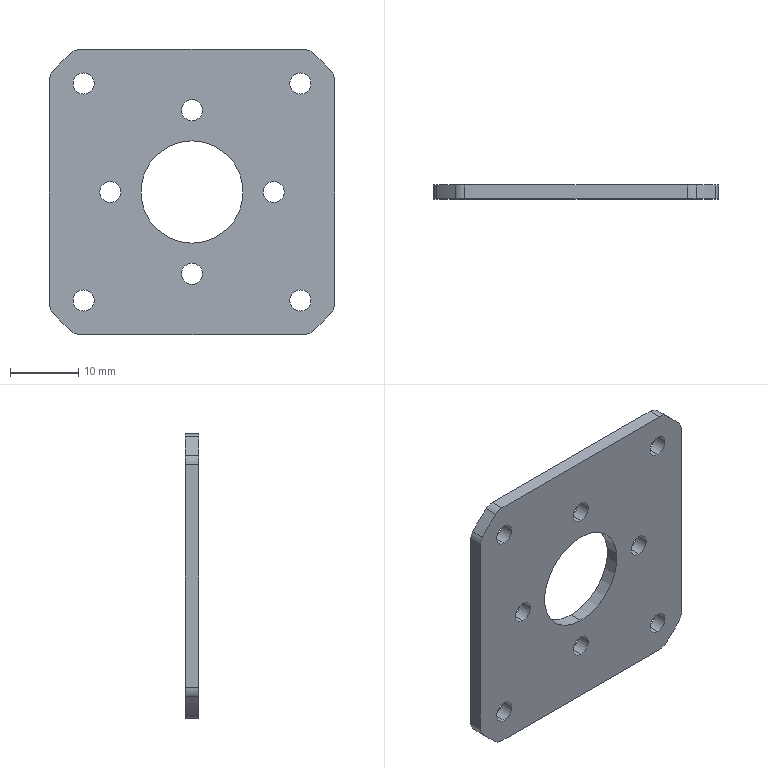Part | SolidWorks | features Extrusion 1, Fillet 1 | 1 solid | 36 faces | box 41.82 x 2 x 41.82 mm | volume 2968 mm3 | cylinder 30 | plane 6 | commonest cylinder face diameters 3.1 x16 4 x8 54 x4 15 x2
STEP:
#1=CARTESIAN_POINT('',(-15.91,2.,-17.46));
#2=VERTEX_POINT('',#1);
#3=CARTESIAN_POINT('',(-15.91,2.,-14.36));
#4=VERTEX_POINT('',#3);
#5=CARTESIAN_POINT('',(-15.91,2.,-15.91));
#6=DIRECTION('',(0.,1.,0.));
#7=DIRECTION('',(0.,0.,1.));
#8=AXIS2_PLACEMENT_3D('',#5,#6,#7);
#9=CIRCLE('',#8,1.55);
#10=EDGE_CURVE('',#2,#4,#9,.T.);
#11=ORIENTED_EDGE('',*,*,#10,.T.);
#12=CARTESIAN_POINT('',(-15.91,0.,-14.36));
#13=VERTEX_POINT('',#12);
#14=CARTESIAN_POINT('',(-15.91,2.,-14.36));
#15=DIRECTION('',(0.,-1.,0.));
#16=VECTOR('',#15,1000.);
#17=LINE('',#14,#16);
#18=EDGE_CURVE('',#4,#13,#17,.T.);
#19=ORIENTED_EDGE('',*,*,#18,.T.);
#20=CARTESIAN_POINT('',(-15.91,0.,-17.46));
#21=VERTEX_POINT('',#20);
#22=CARTESIAN_POINT('',(-15.91,0.,-15.91));
#23=DIRECTION('',(0.,1.,0.));
#24=DIRECTION('',(0.,0.,1.));
#25=AXIS2_PLACEMENT_3D('',#22,#23,#24);
#26=CIRCLE('',#25,1.55);
#27=EDGE_CURVE('',#21,#13,#26,.T.);
#28=ORIENTED_EDGE('',*,*,#27,.F.);
#29=CARTESIAN_POINT('',(-15.91,2.,-17.46));
#30=DIRECTION('',(0.,-1.,0.));
#31=VECTOR('',#30,1000.);
#32=LINE('',#29,#31);
#33=EDGE_CURVE('',#2,#21,#32,.T.);
#34=ORIENTED_EDGE('',*,*,#33,.F.);
#35=EDGE_LOOP('',(#11,#19,#28,#34));
#36=FACE_OUTER_BOUND('',#35,.T.);
#37=CARTESIAN_POINT('',(-15.91,2.,-15.91));
#38=DIRECTION('',(0.,-1.,0.));
#39=DIRECTION('',(0.,0.,-1.));
#40=AXIS2_PLACEMENT_3D('',#37,#38,#39);
#41=CYLINDRICAL_SURFACE('',#40,1.55);
#42=ADVANCED_FACE('',(#36),#41,.F.);
#43=CARTESIAN_POINT('',(0.,2.,-13.55));
#44=VERTEX_POINT('',#43);
#45=CARTESIAN_POINT('',(0.,2.,-10.45));
#46=VERTEX_POINT('',#45);
#47=CARTESIAN_POINT('',(0.,2.,-12.));
#48=DIRECTION('',(0.,1.,0.));
#49=DIRECTION('',(0.,0.,1.));
#50=AXIS2_PLACEMENT_3D('',#47,#48,#49);
#51=CIRCLE('',#50,1.55);
#52=EDGE_CURVE('',#44,#46,#51,.T.);
#53=ORIENTED_EDGE('',*,*,#52,.T.);
#54=CARTESIAN_POINT('',(0.,0.,-10.45));
#55=VERTEX_POINT('',#54);
#56=CARTESIAN_POINT('',(0.,2.,-10.45));
#57=DIRECTION('',(0.,-1.,0.));
#58=VECTOR('',#57,1000.);
#59=LINE('',#56,#58);
#60=EDGE_CURVE('',#46,#55,#59,.T.);
#61=ORIENTED_EDGE('',*,*,#60,.T.);
#62=CARTESIAN_POINT('',(0.,0.,-13.55));
#63=VERTEX_POINT('',#62);
#64=CARTESIAN_POINT('',(0.,0.,-12.));
#65=DIRECTION('',(0.,1.,0.));
#66=DIRECTION('',(0.,0.,1.));
#67=AXIS2_PLACEMENT_3D('',#64,#65,#66);
#68=CIRCLE('',#67,1.55);
#69=EDGE_CURVE('',#63,#55,#68,.T.);
#70=ORIENTED_EDGE('',*,*,#69,.F.);
#71=CARTESIAN_POINT('',(0.,2.,-13.55));
#72=DIRECTION('',(0.,-1.,0.));
#73=VECTOR('',#72,1000.);
#74=LINE('',#71,#73);
#75=EDGE_CURVE('',#44,#63,#74,.T.);
#76=ORIENTED_EDGE('',*,*,#75,.F.);
#77=EDGE_LOOP('',(#53,#61,#70,#76));
#78=FACE_OUTER_BOUND('',#77,.T.);
#79=CARTESIAN_POINT('',(0.,2.,-12.));
#80=DIRECTION('',(0.,-1.,0.));
#81=DIRECTION('',(0.,0.,-1.));
#82=AXIS2_PLACEMENT_3D('',#79,#80,#81);
#83=CYLINDRICAL_SURFACE('',#82,1.55);
#84=ADVANCED_FACE('',(#78),#83,.F.);
#85=CARTESIAN_POINT('',(-15.91,2.,14.36));
#86=VERTEX_POINT('',#85);
#87=CARTESIAN_POINT('',(-15.91,2.,17.46));
#88=VERTEX_POINT('',#87);
#89=CARTESIAN_POINT('',(-15.91,2.,15.91));
#90=DIRECTION('',(0.,1.,0.));
#91=DIRECTION('',(0.,0.,1.));
#92=AXIS2_PLACEMENT_3D('',#89,#90,#91);
#93=CIRCLE('',#92,1.55);
#94=EDGE_CURVE('',#86,#88,#93,.T.);
#95=ORIENTED_EDGE('',*,*,#94,.T.);
#96=CARTESIAN_POINT('',(-15.91,0.,17.46));
#97=VERTEX_POINT('',#96);
#98=CARTESIAN_POINT('',(-15.91,2.,17.46));
#99=DIRECTION('',(0.,-1.,0.));
#100=VECTOR('',#99,1000.);
#101=LINE('',#98,#100);
#102=EDGE_CURVE('',#88,#97,#101,.T.);
#103=ORIENTED_EDGE('',*,*,#102,.T.);
#104=CARTESIAN_POINT('',(-15.91,0.,14.36));
#105=VERTEX_POINT('',#104);
#106=CARTESIAN_POINT('',(-15.91,0.,15.91));
#107=DIRECTION('',(0.,1.,0.));
#108=DIRECTION('',(0.,0.,1.));
#109=AXIS2_PLACEMENT_3D('',#106,#107,#108);
#110=CIRCLE('',#109,1.55);
#111=EDGE_CURVE('',#105,#97,#110,.T.);
#112=ORIENTED_EDGE('',*,*,#111,.F.);
#113=CARTESIAN_POINT('',(-15.91,2.,14.36));
#114=DIRECTION('',(0.,-1.,0.));
#115=VECTOR('',#114,1000.);
#116=LINE('',#113,#115);
#117=EDGE_CURVE('',#86,#105,#116,.T.);
#118=ORIENTED_EDGE('',*,*,#117,.F.);
#119=EDGE_LOOP('',(#95,#103,#112,#118));
#120=FACE_OUTER_BOUND('',#119,.T.);
#121=CARTESIAN_POINT('',(-15.91,2.,15.91));
#122=DIRECTION('',(0.,-1.,0.));
#123=DIRECTION('',(0.,0.,-1.));
#124=AXIS2_PLACEMENT_3D('',#121,#122,#123);
#125=CYLINDRICAL_SURFACE('',#124,1.55);
#126=ADVANCED_FACE('',(#120),#125,.F.);
#127=CARTESIAN_POINT('',(-12.,2.,-1.55));
#128=VERTEX_POINT('',#127);
#129=CARTESIAN_POINT('',(-12.,2.,1.55));
#130=VERTEX_POINT('',#129);
#131=CARTESIAN_POINT('',(-12.,2.,0.));
#132=DIRECTION('',(0.,1.,0.));
#133=DIRECTION('',(0.,0.,1.));
#134=AXIS2_PLACEMENT_3D('',#131,#132,#133);
#135=CIRCLE('',#134,1.55);
#136=EDGE_CURVE('',#128,#130,#135,.T.);
#137=ORIENTED_EDGE('',*,*,#136,.T.);
#138=CARTESIAN_POINT('',(-12.,0.,1.55));
#139=VERTEX_POINT('',#138);
#140=CARTESIAN_POINT('',(-12.,2.,1.55));
#141=DIRECTION('',(0.,-1.,0.));
#142=VECTOR('',#141,1000.);
#143=LINE('',#140,#142);
#144=EDGE_CURVE('',#130,#139,#143,.T.);
#145=ORIENTED_EDGE('',*,*,#144,.T.);
#146=CARTESIAN_POINT('',(-12.,0.,-1.55));
#147=VERTEX_POINT('',#146);
#148=CARTESIAN_POINT('',(-12.,0.,0.));
#149=DIRECTION('',(0.,1.,0.));
#150=DIRECTION('',(0.,0.,1.));
#151=AXIS2_PLACEMENT_3D('',#148,#149,#150);
#152=CIRCLE('',#151,1.55);
#153=EDGE_CURVE('',#147,#139,#152,.T.);
#154=ORIENTED_EDGE('',*,*,#153,.F.);
#155=CARTESIAN_POINT('',(-12.,2.,-1.55));
#156=DIRECTION('',(0.,-1.,0.));
#157=VECTOR('',#156,1000.);
#158=LINE('',#155,#157);
#159=EDGE_CURVE('',#128,#147,#158,.T.);
#160=ORIENTED_EDGE('',*,*,#159,.F.);
#161=EDGE_LOOP('',(#137,#145,#154,#160));
#162=FACE_OUTER_BOUND('',#161,.T.);
#163=CARTESIAN_POINT('',(-12.,2.,0.));
#164=DIRECTION('',(0.,-1.,0.));
#165=DIRECTION('',(0.,0.,-1.));
#166=AXIS2_PLACEMENT_3D('',#163,#164,#165);
#167=CYLINDRICAL_SURFACE('',#166,1.55);
#168=ADVANCED_FACE('',(#162),#167,.F.);
#169=CARTESIAN_POINT('',(15.91,2.,14.36));
#170=VERTEX_POINT('',#169);
#171=CARTESIAN_POINT('',(15.91,2.,17.46));
#172=VERTEX_POINT('',#171);
#173=CARTESIAN_POINT('',(15.91,2.,15.91));
#174=DIRECTION('',(0.,1.,0.));
#175=DIRECTION('',(0.,0.,1.));
#176=AXIS2_PLACEMENT_3D('',#173,#174,#175);
#177=CIRCLE('',#176,1.55);
#178=EDGE_CURVE('',#170,#172,#177,.T.);
#179=ORIENTED_EDGE('',*,*,#178,.T.);
#180=CARTESIAN_POINT('',(15.91,0.,17.46));
#181=VERTEX_POINT('',#180);
#182=CARTESIAN_POINT('',(15.91,2.,17.46));
#183=DIRECTION('',(0.,-1.,0.));
#184=VECTOR('',#183,1000.);
#185=LINE('',#182,#184);
#186=EDGE_CURVE('',#172,#181,#185,.T.);
#187=ORIENTED_EDGE('',*,*,#186,.T.);
#188=CARTESIAN_POINT('',(15.91,0.,14.36));
#189=VERTEX_POINT('',#188);
#190=CARTESIAN_POINT('',(15.91,0.,15.91));
#191=DIRECTION('',(0.,1.,0.));
#192=DIRECTION('',(0.,0.,1.));
#193=AXIS2_PLACEMENT_3D('',#190,#191,#192);
#194=CIRCLE('',#193,1.55);
#195=EDGE_CURVE('',#189,#181,#194,.T.);
#196=ORIENTED_EDGE('',*,*,#195,.F.);
#197=CARTESIAN_POINT('',(15.91,2.,14.36));
#198=DIRECTION('',(0.,-1.,0.));
#199=VECTOR('',#198,1000.);
#200=LINE('',#197,#199);
#201=EDGE_CURVE('',#170,#189,#200,.T.);
#202=ORIENTED_EDGE('',*,*,#201,.F.);
#203=EDGE_LOOP('',(#179,#187,#196,#202));
#204=FACE_OUTER_BOUND('',#203,.T.);
#205=CARTESIAN_POINT('',(15.91,2.,15.91));
#206=DIRECTION('',(0.,-1.,0.));
#207=DIRECTION('',(0.,0.,-1.));
#208=AXIS2_PLACEMENT_3D('',#205,#206,#207);
#209=CYLINDRICAL_SURFACE('',#208,1.55);
#210=ADVANCED_FACE('',(#204),#209,.F.);
#211=CARTESIAN_POINT('',(0.,2.,10.45));
#212=VERTEX_POINT('',#211);
#213=CARTESIAN_POINT('',(0.,2.,13.55));
#214=VERTEX_POINT('',#213);
#215=CARTESIAN_POINT('',(0.,2.,12.));
#216=DIRECTION('',(0.,1.,0.));
#217=DIRECTION('',(0.,0.,1.));
#218=AXIS2_PLACEMENT_3D('',#215,#216,#217);
#219=CIRCLE('',#218,1.55);
#220=EDGE_CURVE('',#212,#214,#219,.T.);
#221=ORIENTED_EDGE('',*,*,#220,.T.);
#222=CARTESIAN_POINT('',(0.,0.,13.55));
#223=VERTEX_POINT('',#222);
#224=CARTESIAN_POINT('',(0.,2.,13.55));
#225=DIRECTION('',(0.,-1.,0.));
#226=VECTOR('',#225,1000.);
#227=LINE('',#224,#226);
#228=EDGE_CURVE('',#214,#223,#227,.T.);
#229=ORIENTED_EDGE('',*,*,#228,.T.);
#230=CARTESIAN_POINT('',(0.,0.,10.45));
#231=VERTEX_POINT('',#230);
#232=CARTESIAN_POINT('',(0.,0.,12.));
#233=DIRECTION('',(0.,1.,0.));
#234=DIRECTION('',(0.,0.,1.));
#235=AXIS2_PLACEMENT_3D('',#232,#233,#234);
#236=CIRCLE('',#235,1.55);
#237=EDGE_CURVE('',#231,#223,#236,.T.);
#238=ORIENTED_EDGE('',*,*,#237,.F.);
#239=CARTESIAN_POINT('',(0.,2.,10.45));
#240=DIRECTION('',(0.,-1.,0.));
#241=VECTOR('',#240,1000.);
#242=LINE('',#239,#241);
#243=EDGE_CURVE('',#212,#231,#242,.T.);
#244=ORIENTED_EDGE('',*,*,#243,.F.);
#245=EDGE_LOOP('',(#221,#229,#238,#244));
#246=FACE_OUTER_BOUND('',#245,.T.);
#247=CARTESIAN_POINT('',(0.,2.,12.));
#248=DIRECTION('',(0.,-1.,0.));
#249=DIRECTION('',(0.,0.,-1.));
#250=AXIS2_PLACEMENT_3D('',#247,#248,#249);
#251=CYLINDRICAL_SURFACE('',#250,1.55);
#252=ADVANCED_FACE('',(#246),#251,.F.);
#253=CARTESIAN_POINT('',(15.91,2.,-17.46));
#254=VERTEX_POINT('',#253);
#255=CARTESIAN_POINT('',(15.91,2.,-14.36));
#256=VERTEX_POINT('',#255);
#257=CARTESIAN_POINT('',(15.91,2.,-15.91));
#258=DIRECTION('',(0.,1.,0.));
#259=DIRECTION('',(0.,0.,1.));
#260=AXIS2_PLACEMENT_3D('',#257,#258,#259);
#261=CIRCLE('',#260,1.55);
#262=EDGE_CURVE('',#254,#256,#261,.T.);
#263=ORIENTED_EDGE('',*,*,#262,.T.);
#264=CARTESIAN_POINT('',(15.91,0.,-14.36));
#265=VERTEX_POINT('',#264);
#266=CARTESIAN_POINT('',(15.91,2.,-14.36));
#267=DIRECTION('',(0.,-1.,0.));
#268=VECTOR('',#267,1000.);
#269=LINE('',#266,#268);
#270=EDGE_CURVE('',#256,#265,#269,.T.);
#271=ORIENTED_EDGE('',*,*,#270,.T.);
#272=CARTESIAN_POINT('',(15.91,0.,-17.46));
#273=VERTEX_POINT('',#272);
#274=CARTESIAN_POINT('',(15.91,0.,-15.91));
#275=DIRECTION('',(0.,1.,0.));
#276=DIRECTION('',(0.,0.,1.));
#277=AXIS2_PLACEMENT_3D('',#274,#275,#276);
#278=CIRCLE('',#277,1.55);
#279=EDGE_CURVE('',#273,#265,#278,.T.);
#280=ORIENTED_EDGE('',*,*,#279,.F.);
#281=CARTESIAN_POINT('',(15.91,2.,-17.46));
#282=DIRECTION('',(0.,-1.,0.));
#283=VECTOR('',#282,1000.);
#284=LINE('',#281,#283);
#285=EDGE_CURVE('',#254,#273,#284,.T.);
#286=ORIENTED_EDGE('',*,*,#285,.F.);
#287=EDGE_LOOP('',(#263,#271,#280,#286));
#288=FACE_OUTER_BOUND('',#287,.T.);
#289=CARTESIAN_POINT('',(15.91,2.,-15.91));
#290=DIRECTION('',(0.,-1.,0.));
#291=DIRECTION('',(0.,0.,-1.));
#292=AXIS2_PLACEMENT_3D('',#289,#290,#291);
#293=CYLINDRICAL_SURFACE('',#292,1.55);
#294=ADVANCED_FACE('',(#288),#293,.F.);
#295=CARTESIAN_POINT('',(12.,2.,-1.55));
#296=VERTEX_POINT('',#295);
#297=CARTESIAN_POINT('',(12.,2.,1.55));
#298=VERTEX_POINT('',#297);
#299=CARTESIAN_POINT('',(12.,2.,0.));
#300=DIRECTION('',(0.,1.,0.));
#301=DIRECTION('',(0.,0.,1.));
#302=AXIS2_PLACEMENT_3D('',#299,#300,#301);
#303=CIRCLE('',#302,1.55);
#304=EDGE_CURVE('',#296,#298,#303,.T.);
#305=ORIENTED_EDGE('',*,*,#304,.T.);
#306=CARTESIAN_POINT('',(12.,0.,1.55));
#307=VERTEX_POINT('',#306);
#308=CARTESIAN_POINT('',(12.,2.,1.55));
#309=DIRECTION('',(0.,-1.,0.));
#310=VECTOR('',#309,1000.);
#311=LINE('',#308,#310);
#312=EDGE_CURVE('',#298,#307,#311,.T.);
#313=ORIENTED_EDGE('',*,*,#312,.T.);
#314=CARTESIAN_POINT('',(12.,0.,-1.55));
#315=VERTEX_POINT('',#314);
#316=CARTESIAN_POINT('',(12.,0.,0.));
#317=DIRECTION('',(0.,1.,0.));
#318=DIRECTION('',(0.,0.,1.));
#319=AXIS2_PLACEMENT_3D('',#316,#317,#318);
#320=CIRCLE('',#319,1.55);
#321=EDGE_CURVE('',#315,#307,#320,.T.);
#322=ORIENTED_EDGE('',*,*,#321,.F.);
#323=CARTESIAN_POINT('',(12.,2.,-1.55));
#324=DIRECTION('',(0.,-1.,0.));
#325=VECTOR('',#324,1000.);
#326=LINE('',#323,#325);
#327=EDGE_CURVE('',#296,#315,#326,.T.);
#328=ORIENTED_EDGE('',*,*,#327,.F.);
#329=EDGE_LOOP('',(#305,#313,#322,#328));
#330=FACE_OUTER_BOUND('',#329,.T.);
#331=CARTESIAN_POINT('',(12.,2.,0.));
#332=DIRECTION('',(0.,-1.,0.));
#333=DIRECTION('',(0.,0.,-1.));
#334=AXIS2_PLACEMENT_3D('',#331,#332,#333);
#335=CYLINDRICAL_SURFACE('',#334,1.55);
#336=ADVANCED_FACE('',(#330),#335,.F.);
#337=CARTESIAN_POINT('',(0.,2.,-7.5));
#338=VERTEX_POINT('',#337);
#339=CARTESIAN_POINT('',(0.,2.,7.5));
#340=VERTEX_POINT('',#339);
#341=CARTESIAN_POINT('',(0.,2.,0.));
#342=DIRECTION('',(0.,1.,0.));
#343=DIRECTION('',(0.,0.,1.));
#344=AXIS2_PLACEMENT_3D('',#341,#342,#343);
#345=CIRCLE('',#344,7.5);
#346=EDGE_CURVE('',#338,#340,#345,.T.);
#347=ORIENTED_EDGE('',*,*,#346,.T.);
#348=CARTESIAN_POINT('',(0.,0.,7.5));
#349=VERTEX_POINT('',#348);
#350=CARTESIAN_POINT('',(0.,2.,7.5));
#351=DIRECTION('',(0.,-1.,0.));
#352=VECTOR('',#351,1000.);
#353=LINE('',#350,#352);
#354=EDGE_CURVE('',#340,#349,#353,.T.);
#355=ORIENTED_EDGE('',*,*,#354,.T.);
#356=CARTESIAN_POINT('',(0.,0.,-7.5));
#357=VERTEX_POINT('',#356);
#358=CARTESIAN_POINT('',(0.,0.,0.));
#359=DIRECTION('',(0.,1.,0.));
#360=DIRECTION('',(0.,0.,1.));
#361=AXIS2_PLACEMENT_3D('',#358,#359,#360);
#362=CIRCLE('',#361,7.5);
#363=EDGE_CURVE('',#357,#349,#362,.T.);
#364=ORIENTED_EDGE('',*,*,#363,.F.);
#365=CARTESIAN_POINT('',(0.,2.,-7.5));
#366=DIRECTION('',(0.,-1.,0.));
#367=VECTOR('',#366,1000.);
#368=LINE('',#365,#367);
#369=EDGE_CURVE('',#338,#357,#368,.T.);
#370=ORIENTED_EDGE('',*,*,#369,.F.);
#371=EDGE_LOOP('',(#347,#355,#364,#370));
#372=FACE_OUTER_BOUND('',#371,.T.);
#373=CARTESIAN_POINT('',(0.,2.,0.));
#374=DIRECTION('',(0.,-1.,0.));
#375=DIRECTION('',(0.,0.,-1.));
#376=AXIS2_PLACEMENT_3D('',#373,#374,#375);
#377=CYLINDRICAL_SURFACE('',#376,7.5);
#378=ADVANCED_FACE('',(#372),#377,.F.);
#379=ORIENTED_EDGE('',*,*,#52,.F.);
#380=CARTESIAN_POINT('',(0.,2.,-12.));
#381=DIRECTION('',(0.,1.,0.));
#382=DIRECTION('',(0.,0.,1.));
#383=AXIS2_PLACEMENT_3D('',#380,#381,#382);
#384=CIRCLE('',#383,1.55);
#385=EDGE_CURVE('',#46,#44,#384,.T.);
#386=ORIENTED_EDGE('',*,*,#385,.F.);
#387=EDGE_LOOP('',(#379,#386));
#388=FACE_BOUND('',#387,.T.);
#389=ORIENTED_EDGE('',*,*,#136,.F.);
#390=CARTESIAN_POINT('',(-12.,2.,0.));
#391=DIRECTION('',(0.,1.,0.));
#392=DIRECTION('',(0.,0.,1.));
#393=AXIS2_PLACEMENT_3D('',#390,#391,#392);
#394=CIRCLE('',#393,1.55);
#395=EDGE_CURVE('',#130,#128,#394,.T.);
#396=ORIENTED_EDGE('',*,*,#395,.F.);
#397=EDGE_LOOP('',(#389,#396));
#398=FACE_BOUND('',#397,.T.);
#399=ORIENTED_EDGE('',*,*,#220,.F.);
#400=CARTESIAN_POINT('',(0.,2.,12.));
#401=DIRECTION('',(0.,1.,0.));
#402=DIRECTION('',(0.,0.,1.));
#403=AXIS2_PLACEMENT_3D('',#400,#401,#402);
#404=CIRCLE('',#403,1.55);
#405=EDGE_CURVE('',#214,#212,#404,.T.);
#406=ORIENTED_EDGE('',*,*,#405,.F.);
#407=EDGE_LOOP('',(#399,#406));
#408=FACE_BOUND('',#407,.T.);
#409=ORIENTED_EDGE('',*,*,#304,.F.);
#410=CARTESIAN_POINT('',(12.,2.,0.));
#411=DIRECTION('',(0.,1.,0.));
#412=DIRECTION('',(0.,0.,1.));
#413=AXIS2_PLACEMENT_3D('',#410,#411,#412);
#414=CIRCLE('',#413,1.55);
#415=EDGE_CURVE('',#298,#296,#414,.T.);
#416=ORIENTED_EDGE('',*,*,#415,.F.);
#417=EDGE_LOOP('',(#409,#416));
#418=FACE_BOUND('',#417,.T.);
#419=CARTESIAN_POINT('',(-16.353,2.,20.91));
#420=VERTEX_POINT('',#419);
#421=CARTESIAN_POINT('',(16.353,2.,20.91));
#422=VERTEX_POINT('',#421);
#423=CARTESIAN_POINT('',(17.081,2.,20.91));
#424=DIRECTION('',(1.,0.,0.));
#425=VECTOR('',#424,1000.);
#426=LINE('',#423,#425);
#427=EDGE_CURVE('',#420,#422,#426,.T.);
#428=ORIENTED_EDGE('',*,*,#427,.T.);
#429=CARTESIAN_POINT('',(17.661,2.,20.423));
#430=VERTEX_POINT('',#429);
#431=CARTESIAN_POINT('',(16.353,2.,18.91));
#432=DIRECTION('',(0.,1.,0.));
#433=DIRECTION('',(0.,0.,1.));
#434=AXIS2_PLACEMENT_3D('',#431,#432,#433);
#435=CIRCLE('',#434,2.);
#436=EDGE_CURVE('',#422,#430,#435,.T.);
#437=ORIENTED_EDGE('',*,*,#436,.T.);
#438=CARTESIAN_POINT('',(20.423,2.,17.661));
#439=VERTEX_POINT('',#438);
#440=CARTESIAN_POINT('',(0.,2.,0.));
#441=DIRECTION('',(0.,1.,0.));
#442=DIRECTION('',(0.,0.,1.));
#443=AXIS2_PLACEMENT_3D('',#440,#441,#442);
#444=CIRCLE('',#443,27.);
#445=EDGE_CURVE('',#430,#439,#444,.T.);
#446=ORIENTED_EDGE('',*,*,#445,.T.);
#447=CARTESIAN_POINT('',(20.91,2.,16.353));
#448=VERTEX_POINT('',#447);
#449=CARTESIAN_POINT('',(18.91,2.,16.353));
#450=DIRECTION('',(0.,1.,0.));
#451=DIRECTION('',(0.,0.,1.));
#452=AXIS2_PLACEMENT_3D('',#449,#450,#451);
#453=CIRCLE('',#452,2.);
#454=EDGE_CURVE('',#439,#448,#453,.T.);
#455=ORIENTED_EDGE('',*,*,#454,.T.);
#456=CARTESIAN_POINT('',(20.91,2.,-16.353));
#457=VERTEX_POINT('',#456);
#458=CARTESIAN_POINT('',(20.91,2.,-17.081));
#459=DIRECTION('',(0.,0.,-1.));
#460=VECTOR('',#459,1000.);
#461=LINE('',#458,#460);
#462=EDGE_CURVE('',#448,#457,#461,.T.);
#463=ORIENTED_EDGE('',*,*,#462,.T.);
#464=CARTESIAN_POINT('',(20.423,2.,-17.661));
#465=VERTEX_POINT('',#464);
#466=CARTESIAN_POINT('',(18.91,2.,-16.353));
#467=DIRECTION('',(0.,1.,0.));
#468=DIRECTION('',(0.,0.,1.));
#469=AXIS2_PLACEMENT_3D('',#466,#467,#468);
#470=CIRCLE('',#469,2.);
#471=EDGE_CURVE('',#457,#465,#470,.T.);
#472=ORIENTED_EDGE('',*,*,#471,.T.);
#473=CARTESIAN_POINT('',(17.661,2.,-20.423));
#474=VERTEX_POINT('',#473);
#475=CARTESIAN_POINT('',(0.,2.,0.));
#476=DIRECTION('',(0.,1.,0.));
#477=DIRECTION('',(0.,0.,1.));
#478=AXIS2_PLACEMENT_3D('',#475,#476,#477);
#479=CIRCLE('',#478,27.);
#480=EDGE_CURVE('',#465,#474,#479,.T.);
#481=ORIENTED_EDGE('',*,*,#480,.T.);
#482=CARTESIAN_POINT('',(16.353,2.,-20.91));
#483=VERTEX_POINT('',#482);
#484=CARTESIAN_POINT('',(16.353,2.,-18.91));
#485=DIRECTION('',(0.,1.,0.));
#486=DIRECTION('',(0.,0.,1.));
#487=AXIS2_PLACEMENT_3D('',#484,#485,#486);
#488=CIRCLE('',#487,2.);
#489=EDGE_CURVE('',#474,#483,#488,.T.);
#490=ORIENTED_EDGE('',*,*,#489,.T.);
#491=CARTESIAN_POINT('',(-16.353,2.,-20.91));
#492=VERTEX_POINT('',#491);
#493=CARTESIAN_POINT('',(17.081,2.,-20.91));
#494=DIRECTION('',(-1.,0.,0.));
#495=VECTOR('',#494,1000.);
#496=LINE('',#493,#495);
#497=EDGE_CURVE('',#483,#492,#496,.T.);
#498=ORIENTED_EDGE('',*,*,#497,.T.);
#499=CARTESIAN_POINT('',(-17.661,2.,-20.423));
#500=VERTEX_POINT('',#499);
#501=CARTESIAN_POINT('',(-16.353,2.,-18.91));
#502=DIRECTION('',(0.,1.,0.));
#503=DIRECTION('',(0.,0.,1.));
#504=AXIS2_PLACEMENT_3D('',#501,#502,#503);
#505=CIRCLE('',#504,2.);
#506=EDGE_CURVE('',#492,#500,#505,.T.);
#507=ORIENTED_EDGE('',*,*,#506,.T.);
#508=CARTESIAN_POINT('',(-20.423,2.,-17.661));
#509=VERTEX_POINT('',#508);
#510=CARTESIAN_POINT('',(0.,2.,0.));
#511=DIRECTION('',(0.,1.,0.));
#512=DIRECTION('',(0.,0.,1.));
#513=AXIS2_PLACEMENT_3D('',#510,#511,#512);
#514=CIRCLE('',#513,27.);
#515=EDGE_CURVE('',#500,#509,#514,.T.);
#516=ORIENTED_EDGE('',*,*,#515,.T.);
#517=CARTESIAN_POINT('',(-20.91,2.,-16.353));
#518=VERTEX_POINT('',#517);
#519=CARTESIAN_POINT('',(-18.91,2.,-16.353));
#520=DIRECTION('',(0.,1.,0.));
#521=DIRECTION('',(0.,0.,1.));
#522=AXIS2_PLACEMENT_3D('',#519,#520,#521);
#523=CIRCLE('',#522,2.);
#524=EDGE_CURVE('',#509,#518,#523,.T.);
#525=ORIENTED_EDGE('',*,*,#524,.T.);
#526=CARTESIAN_POINT('',(-20.91,2.,16.353));
#527=VERTEX_POINT('',#526);
#528=CARTESIAN_POINT('',(-20.91,2.,-17.081));
#529=DIRECTION('',(0.,0.,1.));
#530=VECTOR('',#529,1000.);
#531=LINE('',#528,#530);
#532=EDGE_CURVE('',#518,#527,#531,.T.);
#533=ORIENTED_EDGE('',*,*,#532,.T.);
#534=CARTESIAN_POINT('',(-20.423,2.,17.661));
#535=VERTEX_POINT('',#534);
#536=CARTESIAN_POINT('',(-18.91,2.,16.353));
#537=DIRECTION('',(0.,1.,0.));
#538=DIRECTION('',(0.,0.,1.));
#539=AXIS2_PLACEMENT_3D('',#536,#537,#538);
#540=CIRCLE('',#539,2.);
#541=EDGE_CURVE('',#527,#535,#540,.T.);
#542=ORIENTED_EDGE('',*,*,#541,.T.);
#543=CARTESIAN_POINT('',(-17.661,2.,20.423));
#544=VERTEX_POINT('',#543);
#545=CARTESIAN_POINT('',(0.,2.,0.));
#546=DIRECTION('',(0.,1.,0.));
#547=DIRECTION('',(0.,0.,1.));
#548=AXIS2_PLACEMENT_3D('',#545,#546,#547);
#549=CIRCLE('',#548,27.);
#550=EDGE_CURVE('',#535,#544,#549,.T.);
#551=ORIENTED_EDGE('',*,*,#550,.T.);
#552=CARTESIAN_POINT('',(-16.353,2.,18.91));
#553=DIRECTION('',(0.,1.,0.));
#554=DIRECTION('',(0.,0.,1.));
#555=AXIS2_PLACEMENT_3D('',#552,#553,#554);
#556=CIRCLE('',#555,2.);
#557=EDGE_CURVE('',#544,#420,#556,.T.);
#558=ORIENTED_EDGE('',*,*,#557,.T.);
#559=EDGE_LOOP('',(#428,#437,#446,#455,#463,#472,#481,#490,#498,#507,#516,#525,#533,#542,#551,#558));
#560=FACE_OUTER_BOUND('',#559,.T.);
#561=ORIENTED_EDGE('',*,*,#346,.F.);
#562=CARTESIAN_POINT('',(0.,2.,0.));
#563=DIRECTION('',(0.,1.,0.));
#564=DIRECTION('',(0.,0.,1.));
#565=AXIS2_PLACEMENT_3D('',#562,#563,#564);
#566=CIRCLE('',#565,7.5);
#567=EDGE_CURVE('',#340,#338,#566,.T.);
#568=ORIENTED_EDGE('',*,*,#567,.F.);
#569=EDGE_LOOP('',(#561,#568));
#570=FACE_BOUND('',#569,.T.);
#571=ORIENTED_EDGE('',*,*,#262,.F.);
#572=CARTESIAN_POINT('',(15.91,2.,-15.91));
#573=DIRECTION('',(0.,1.,0.));
#574=DIRECTION('',(0.,0.,1.));
#575=AXIS2_PLACEMENT_3D('',#572,#573,#574);
#576=CIRCLE('',#575,1.55);
#577=EDGE_CURVE('',#256,#254,#576,.T.);
#578=ORIENTED_EDGE('',*,*,#577,.F.);
#579=EDGE_LOOP('',(#571,#578));
#580=FACE_BOUND('',#579,.T.);
#581=ORIENTED_EDGE('',*,*,#178,.F.);
#582=CARTESIAN_POINT('',(15.91,2.,15.91));
#583=DIRECTION('',(0.,1.,0.));
#584=DIRECTION('',(0.,0.,1.));
#585=AXIS2_PLACEMENT_3D('',#582,#583,#584);
#586=CIRCLE('',#585,1.55);
#587=EDGE_CURVE('',#172,#170,#586,.T.);
#588=ORIENTED_EDGE('',*,*,#587,.F.);
#589=EDGE_LOOP('',(#581,#588));
#590=FACE_BOUND('',#589,.T.);
#591=ORIENTED_EDGE('',*,*,#94,.F.);
#592=CARTESIAN_POINT('',(-15.91,2.,15.91));
#593=DIRECTION('',(0.,1.,0.));
#594=DIRECTION('',(0.,0.,1.));
#595=AXIS2_PLACEMENT_3D('',#592,#593,#594);
#596=CIRCLE('',#595,1.55);
#597=EDGE_CURVE('',#88,#86,#596,.T.);
#598=ORIENTED_EDGE('',*,*,#597,.F.);
#599=EDGE_LOOP('',(#591,#598));
#600=FACE_BOUND('',#599,.T.);
#601=ORIENTED_EDGE('',*,*,#10,.F.);
#602=CARTESIAN_POINT('',(-15.91,2.,-15.91));
#603=DIRECTION('',(0.,1.,0.));
#604=DIRECTION('',(0.,0.,1.));
#605=AXIS2_PLACEMENT_3D('',#602,#603,#604);
#606=CIRCLE('',#605,1.55);
#607=EDGE_CURVE('',#4,#2,#606,.T.);
#608=ORIENTED_EDGE('',*,*,#607,.F.);
#609=EDGE_LOOP('',(#601,#608));
#610=FACE_BOUND('',#609,.T.);
#611=CARTESIAN_POINT('',(0.,2.,0.));
#612=DIRECTION('',(0.,1.,0.));
#613=DIRECTION('',(0.,0.,1.));
#614=AXIS2_PLACEMENT_3D('',#611,#612,#613);
#615=PLANE('',#614);
#616=ADVANCED_FACE('',(#388,#398,#408,#418,#560,#570,#580,#590,#600,#610),#615,.T.);
#617=CARTESIAN_POINT('',(17.661,0.,20.423));
#618=VERTEX_POINT('',#617);
#619=CARTESIAN_POINT('',(20.423,0.,17.661));
#620=VERTEX_POINT('',#619);
#621=CARTESIAN_POINT('',(0.,0.,0.));
#622=DIRECTION('',(0.,1.,0.));
#623=DIRECTION('',(0.,0.,1.));
#624=AXIS2_PLACEMENT_3D('',#621,#622,#623);
#625=CIRCLE('',#624,27.);
#626=EDGE_CURVE('',#618,#620,#625,.T.);
#627=ORIENTED_EDGE('',*,*,#626,.F.);
#628=CARTESIAN_POINT('',(16.353,0.,20.91));
#629=VERTEX_POINT('',#628);
#630=CARTESIAN_POINT('',(16.353,0.,18.91));
#631=DIRECTION('',(0.,-1.,0.));
#632=DIRECTION('',(0.,0.,1.));
#633=AXIS2_PLACEMENT_3D('',#630,#631,#632);
#634=CIRCLE('',#633,2.);
#635=EDGE_CURVE('',#618,#629,#634,.T.);
#636=ORIENTED_EDGE('',*,*,#635,.T.);
#637=CARTESIAN_POINT('',(-16.353,0.,20.91));
#638=VERTEX_POINT('',#637);
#639=CARTESIAN_POINT('',(17.081,0.,20.91));
#640=DIRECTION('',(1.,0.,0.));
#641=VECTOR('',#640,1000.);
#642=LINE('',#639,#641);
#643=EDGE_CURVE('',#638,#629,#642,.T.);
#644=ORIENTED_EDGE('',*,*,#643,.F.);
#645=CARTESIAN_POINT('',(-17.661,0.,20.423));
#646=VERTEX_POINT('',#645);
#647=CARTESIAN_POINT('',(-16.353,0.,18.91));
#648=DIRECTION('',(0.,-1.,0.));
#649=DIRECTION('',(0.,0.,1.));
#650=AXIS2_PLACEMENT_3D('',#647,#648,#649);
#651=CIRCLE('',#650,2.);
#652=EDGE_CURVE('',#638,#646,#651,.T.);
#653=ORIENTED_EDGE('',*,*,#652,.T.);
#654=CARTESIAN_POINT('',(-20.423,0.,17.661));
#655=VERTEX_POINT('',#654);
#656=CARTESIAN_POINT('',(0.,0.,0.));
#657=DIRECTION('',(0.,1.,0.));
#658=DIRECTION('',(0.,0.,1.));
#659=AXIS2_PLACEMENT_3D('',#656,#657,#658);
#660=CIRCLE('',#659,27.);
#661=EDGE_CURVE('',#655,#646,#660,.T.);
#662=ORIENTED_EDGE('',*,*,#661,.F.);
#663=CARTESIAN_POINT('',(-20.91,0.,16.353));
#664=VERTEX_POINT('',#663);
#665=CARTESIAN_POINT('',(-18.91,0.,16.353));
#666=DIRECTION('',(0.,-1.,0.));
#667=DIRECTION('',(0.,0.,1.));
#668=AXIS2_PLACEMENT_3D('',#665,#666,#667);
#669=CIRCLE('',#668,2.);
#670=EDGE_CURVE('',#655,#664,#669,.T.);
#671=ORIENTED_EDGE('',*,*,#670,.T.);
#672=CARTESIAN_POINT('',(-20.91,0.,-16.353));
#673=VERTEX_POINT('',#672);
#674=CARTESIAN_POINT('',(-20.91,0.,-17.081));
#675=DIRECTION('',(0.,0.,1.));
#676=VECTOR('',#675,1000.);
#677=LINE('',#674,#676);
#678=EDGE_CURVE('',#673,#664,#677,.T.);
#679=ORIENTED_EDGE('',*,*,#678,.F.);
#680=CARTESIAN_POINT('',(-20.423,0.,-17.661));
#681=VERTEX_POINT('',#680);
#682=CARTESIAN_POINT('',(-18.91,0.,-16.353));
#683=DIRECTION('',(0.,-1.,0.));
#684=DIRECTION('',(0.,0.,1.));
#685=AXIS2_PLACEMENT_3D('',#682,#683,#684);
#686=CIRCLE('',#685,2.);
#687=EDGE_CURVE('',#673,#681,#686,.T.);
#688=ORIENTED_EDGE('',*,*,#687,.T.);
#689=CARTESIAN_POINT('',(-17.661,0.,-20.423));
#690=VERTEX_POINT('',#689);
#691=CARTESIAN_POINT('',(0.,0.,0.));
#692=DIRECTION('',(0.,1.,0.));
#693=DIRECTION('',(0.,0.,1.));
#694=AXIS2_PLACEMENT_3D('',#691,#692,#693);
#695=CIRCLE('',#694,27.);
#696=EDGE_CURVE('',#690,#681,#695,.T.);
#697=ORIENTED_EDGE('',*,*,#696,.F.);
#698=CARTESIAN_POINT('',(-16.353,0.,-20.91));
#699=VERTEX_POINT('',#698);
#700=CARTESIAN_POINT('',(-16.353,0.,-18.91));
#701=DIRECTION('',(0.,-1.,0.));
#702=DIRECTION('',(0.,0.,1.));
#703=AXIS2_PLACEMENT_3D('',#700,#701,#702);
#704=CIRCLE('',#703,2.);
#705=EDGE_CURVE('',#690,#699,#704,.T.);
#706=ORIENTED_EDGE('',*,*,#705,.T.);
#707=CARTESIAN_POINT('',(16.353,0.,-20.91));
#708=VERTEX_POINT('',#707);
#709=CARTESIAN_POINT('',(17.081,0.,-20.91));
#710=DIRECTION('',(-1.,0.,0.));
#711=VECTOR('',#710,1000.);
#712=LINE('',#709,#711);
#713=EDGE_CURVE('',#708,#699,#712,.T.);
#714=ORIENTED_EDGE('',*,*,#713,.F.);
#715=CARTESIAN_POINT('',(17.661,0.,-20.423));
#716=VERTEX_POINT('',#715);
#717=CARTESIAN_POINT('',(16.353,0.,-18.91));
#718=DIRECTION('',(0.,-1.,0.));
#719=DIRECTION('',(0.,0.,1.));
#720=AXIS2_PLACEMENT_3D('',#717,#718,#719);
#721=CIRCLE('',#720,2.);
#722=EDGE_CURVE('',#708,#716,#721,.T.);
#723=ORIENTED_EDGE('',*,*,#722,.T.);
#724=CARTESIAN_POINT('',(20.423,0.,-17.661));
#725=VERTEX_POINT('',#724);
#726=CARTESIAN_POINT('',(0.,0.,0.));
#727=DIRECTION('',(0.,1.,0.));
#728=DIRECTION('',(0.,0.,1.));
#729=AXIS2_PLACEMENT_3D('',#726,#727,#728);
#730=CIRCLE('',#729,27.);
#731=EDGE_CURVE('',#725,#716,#730,.T.);
#732=ORIENTED_EDGE('',*,*,#731,.F.);
#733=CARTESIAN_POINT('',(20.91,0.,-16.353));
#734=VERTEX_POINT('',#733);
#735=CARTESIAN_POINT('',(18.91,0.,-16.353));
#736=DIRECTION('',(0.,-1.,0.));
#737=DIRECTION('',(0.,0.,1.));
#738=AXIS2_PLACEMENT_3D('',#735,#736,#737);
#739=CIRCLE('',#738,2.);
#740=EDGE_CURVE('',#725,#734,#739,.T.);
#741=ORIENTED_EDGE('',*,*,#740,.T.);
#742=CARTESIAN_POINT('',(20.91,0.,16.353));
#743=VERTEX_POINT('',#742);
#744=CARTESIAN_POINT('',(20.91,0.,-17.081));
#745=DIRECTION('',(0.,0.,-1.));
#746=VECTOR('',#745,1000.);
#747=LINE('',#744,#746);
#748=EDGE_CURVE('',#743,#734,#747,.T.);
#749=ORIENTED_EDGE('',*,*,#748,.F.);
#750=CARTESIAN_POINT('',(18.91,0.,16.353));
#751=DIRECTION('',(0.,-1.,0.));
#752=DIRECTION('',(0.,0.,1.));
#753=AXIS2_PLACEMENT_3D('',#750,#751,#752);
#754=CIRCLE('',#753,2.);
#755=EDGE_CURVE('',#743,#620,#754,.T.);
#756=ORIENTED_EDGE('',*,*,#755,.T.);
#757=EDGE_LOOP('',(#627,#636,#644,#653,#662,#671,#679,#688,#697,#706,#714,#723,#732,#741,#749,#756));
#758=FACE_OUTER_BOUND('',#757,.T.);
#759=ORIENTED_EDGE('',*,*,#363,.T.);
#760=CARTESIAN_POINT('',(0.,0.,0.));
#761=DIRECTION('',(0.,1.,0.));
#762=DIRECTION('',(0.,0.,1.));
#763=AXIS2_PLACEMENT_3D('',#760,#761,#762);
#764=CIRCLE('',#763,7.5);
#765=EDGE_CURVE('',#349,#357,#764,.T.);
#766=ORIENTED_EDGE('',*,*,#765,.T.);
#767=EDGE_LOOP('',(#759,#766));
#768=FACE_BOUND('',#767,.T.);
#769=ORIENTED_EDGE('',*,*,#321,.T.);
#770=CARTESIAN_POINT('',(12.,0.,0.));
#771=DIRECTION('',(0.,1.,0.));
#772=DIRECTION('',(0.,0.,1.));
#773=AXIS2_PLACEMENT_3D('',#770,#771,#772);
#774=CIRCLE('',#773,1.55);
#775=EDGE_CURVE('',#307,#315,#774,.T.);
#776=ORIENTED_EDGE('',*,*,#775,.T.);
#777=EDGE_LOOP('',(#769,#776));
#778=FACE_BOUND('',#777,.T.);
#779=ORIENTED_EDGE('',*,*,#279,.T.);
#780=CARTESIAN_POINT('',(15.91,0.,-15.91));
#781=DIRECTION('',(0.,1.,0.));
#782=DIRECTION('',(0.,0.,1.));
#783=AXIS2_PLACEMENT_3D('',#780,#781,#782);
#784=CIRCLE('',#783,1.55);
#785=EDGE_CURVE('',#265,#273,#784,.T.);
#786=ORIENTED_EDGE('',*,*,#785,.T.);
#787=EDGE_LOOP('',(#779,#786));
#788=FACE_BOUND('',#787,.T.);
#789=ORIENTED_EDGE('',*,*,#237,.T.);
#790=CARTESIAN_POINT('',(0.,0.,12.));
#791=DIRECTION('',(0.,1.,0.));
#792=DIRECTION('',(0.,0.,1.));
#793=AXIS2_PLACEMENT_3D('',#790,#791,#792);
#794=CIRCLE('',#793,1.55);
#795=EDGE_CURVE('',#223,#231,#794,.T.);
#796=ORIENTED_EDGE('',*,*,#795,.T.);
#797=EDGE_LOOP('',(#789,#796));
#798=FACE_BOUND('',#797,.T.);
#799=ORIENTED_EDGE('',*,*,#195,.T.);
#800=CARTESIAN_POINT('',(15.91,0.,15.91));
#801=DIRECTION('',(0.,1.,0.));
#802=DIRECTION('',(0.,0.,1.));
#803=AXIS2_PLACEMENT_3D('',#800,#801,#802);
#804=CIRCLE('',#803,1.55);
#805=EDGE_CURVE('',#181,#189,#804,.T.);
#806=ORIENTED_EDGE('',*,*,#805,.T.);
#807=EDGE_LOOP('',(#799,#806));
#808=FACE_BOUND('',#807,.T.);
#809=ORIENTED_EDGE('',*,*,#153,.T.);
#810=CARTESIAN_POINT('',(-12.,0.,0.));
#811=DIRECTION('',(0.,1.,0.));
#812=DIRECTION('',(0.,0.,1.));
#813=AXIS2_PLACEMENT_3D('',#810,#811,#812);
#814=CIRCLE('',#813,1.55);
#815=EDGE_CURVE('',#139,#147,#814,.T.);
#816=ORIENTED_EDGE('',*,*,#815,.T.);
#817=EDGE_LOOP('',(#809,#816));
#818=FACE_BOUND('',#817,.T.);
#819=ORIENTED_EDGE('',*,*,#111,.T.);
#820=CARTESIAN_POINT('',(-15.91,0.,15.91));
#821=DIRECTION('',(0.,1.,0.));
#822=DIRECTION('',(0.,0.,1.));
#823=AXIS2_PLACEMENT_3D('',#820,#821,#822);
#824=CIRCLE('',#823,1.55);
#825=EDGE_CURVE('',#97,#105,#824,.T.);
#826=ORIENTED_EDGE('',*,*,#825,.T.);
#827=EDGE_LOOP('',(#819,#826));
#828=FACE_BOUND('',#827,.T.);
#829=ORIENTED_EDGE('',*,*,#69,.T.);
#830=CARTESIAN_POINT('',(0.,0.,-12.));
#831=DIRECTION('',(0.,1.,0.));
#832=DIRECTION('',(0.,0.,1.));
#833=AXIS2_PLACEMENT_3D('',#830,#831,#832);
#834=CIRCLE('',#833,1.55);
#835=EDGE_CURVE('',#55,#63,#834,.T.);
#836=ORIENTED_EDGE('',*,*,#835,.T.);
#837=EDGE_LOOP('',(#829,#836));
#838=FACE_BOUND('',#837,.T.);
#839=ORIENTED_EDGE('',*,*,#27,.T.);
#840=CARTESIAN_POINT('',(-15.91,0.,-15.91));
#841=DIRECTION('',(0.,1.,0.));
#842=DIRECTION('',(0.,0.,1.));
#843=AXIS2_PLACEMENT_3D('',#840,#841,#842);
#844=CIRCLE('',#843,1.55);
#845=EDGE_CURVE('',#13,#21,#844,.T.);
#846=ORIENTED_EDGE('',*,*,#845,.T.);
#847=EDGE_LOOP('',(#839,#846));
#848=FACE_BOUND('',#847,.T.);
#849=CARTESIAN_POINT('',(0.,0.,0.));
#850=DIRECTION('',(0.,1.,0.));
#851=DIRECTION('',(0.,0.,1.));
#852=AXIS2_PLACEMENT_3D('',#849,#850,#851);
#853=PLANE('',#852);
#854=ADVANCED_FACE('',(#758,#768,#778,#788,#798,#808,#818,#828,#838,#848),#853,.F.);
#855=ORIENTED_EDGE('',*,*,#445,.F.);
#856=CARTESIAN_POINT('',(17.661,2.,20.423));
#857=DIRECTION('',(0.,-1.,0.));
#858=VECTOR('',#857,1000.);
#859=LINE('',#856,#858);
#860=EDGE_CURVE('',#430,#618,#859,.T.);
#861=ORIENTED_EDGE('',*,*,#860,.T.);
#862=ORIENTED_EDGE('',*,*,#626,.T.);
#863=CARTESIAN_POINT('',(20.423,2.,17.661));
#864=DIRECTION('',(0.,1.,0.));
#865=VECTOR('',#864,1000.);
#866=LINE('',#863,#865);
#867=EDGE_CURVE('',#620,#439,#866,.T.);
#868=ORIENTED_EDGE('',*,*,#867,.T.);
#869=EDGE_LOOP('',(#855,#861,#862,#868));
#870=FACE_OUTER_BOUND('',#869,.T.);
#871=CARTESIAN_POINT('',(0.,2.,0.));
#872=DIRECTION('',(0.,-1.,0.));
#873=DIRECTION('',(0.,0.,-1.));
#874=AXIS2_PLACEMENT_3D('',#871,#872,#873);
#875=CYLINDRICAL_SURFACE('',#874,27.);
#876=ADVANCED_FACE('',(#870),#875,.T.);
#877=ORIENTED_EDGE('',*,*,#748,.T.);
#878=CARTESIAN_POINT('',(20.91,2.,-16.353));
#879=DIRECTION('',(0.,1.,0.));
#880=VECTOR('',#879,1000.);
#881=LINE('',#878,#880);
#882=EDGE_CURVE('',#734,#457,#881,.T.);
#883=ORIENTED_EDGE('',*,*,#882,.T.);
#884=ORIENTED_EDGE('',*,*,#462,.F.);
#885=CARTESIAN_POINT('',(20.91,2.,16.353));
#886=DIRECTION('',(0.,-1.,0.));
#887=VECTOR('',#886,1000.);
#888=LINE('',#885,#887);
#889=EDGE_CURVE('',#448,#743,#888,.T.);
#890=ORIENTED_EDGE('',*,*,#889,.T.);
#891=EDGE_LOOP('',(#877,#883,#884,#890));
#892=FACE_OUTER_BOUND('',#891,.T.);
#893=CARTESIAN_POINT('',(20.91,2.,-17.081));
#894=DIRECTION('',(-1.,0.,0.));
#895=DIRECTION('',(0.,0.,1.));
#896=AXIS2_PLACEMENT_3D('',#893,#894,#895);
#897=PLANE('',#896);
#898=ADVANCED_FACE('',(#892),#897,.F.);
#899=ORIENTED_EDGE('',*,*,#731,.T.);
#900=CARTESIAN_POINT('',(17.661,2.,-20.423));
#901=DIRECTION('',(0.,1.,0.));
#902=VECTOR('',#901,1000.);
#903=LINE('',#900,#902);
#904=EDGE_CURVE('',#716,#474,#903,.T.);
#905=ORIENTED_EDGE('',*,*,#904,.T.);
#906=ORIENTED_EDGE('',*,*,#480,.F.);
#907=CARTESIAN_POINT('',(20.423,2.,-17.661));
#908=DIRECTION('',(0.,-1.,0.));
#909=VECTOR('',#908,1000.);
#910=LINE('',#907,#909);
#911=EDGE_CURVE('',#465,#725,#910,.T.);
#912=ORIENTED_EDGE('',*,*,#911,.T.);
#913=EDGE_LOOP('',(#899,#905,#906,#912));
#914=FACE_OUTER_BOUND('',#913,.T.);
#915=CARTESIAN_POINT('',(0.,2.,0.));
#916=DIRECTION('',(0.,-1.,0.));
#917=DIRECTION('',(0.,0.,-1.));
#918=AXIS2_PLACEMENT_3D('',#915,#916,#917);
#919=CYLINDRICAL_SURFACE('',#918,27.);
#920=ADVANCED_FACE('',(#914),#919,.T.);
#921=ORIENTED_EDGE('',*,*,#713,.T.);
#922=CARTESIAN_POINT('',(-16.353,2.,-20.91));
#923=DIRECTION('',(0.,1.,0.));
#924=VECTOR('',#923,1000.);
#925=LINE('',#922,#924);
#926=EDGE_CURVE('',#699,#492,#925,.T.);
#927=ORIENTED_EDGE('',*,*,#926,.T.);
#928=ORIENTED_EDGE('',*,*,#497,.F.);
#929=CARTESIAN_POINT('',(16.353,2.,-20.91));
#930=DIRECTION('',(0.,-1.,0.));
#931=VECTOR('',#930,1000.);
#932=LINE('',#929,#931);
#933=EDGE_CURVE('',#483,#708,#932,.T.);
#934=ORIENTED_EDGE('',*,*,#933,.T.);
#935=EDGE_LOOP('',(#921,#927,#928,#934));
#936=FACE_OUTER_BOUND('',#935,.T.);
#937=CARTESIAN_POINT('',(17.081,2.,-20.91));
#938=DIRECTION('',(0.,0.,1.));
#939=DIRECTION('',(1.,0.,0.));
#940=AXIS2_PLACEMENT_3D('',#937,#938,#939);
#941=PLANE('',#940);
#942=ADVANCED_FACE('',(#936),#941,.F.);
#943=ORIENTED_EDGE('',*,*,#515,.F.);
#944=CARTESIAN_POINT('',(-17.661,2.,-20.423));
#945=DIRECTION('',(0.,-1.,0.));
#946=VECTOR('',#945,1000.);
#947=LINE('',#944,#946);
#948=EDGE_CURVE('',#500,#690,#947,.T.);
#949=ORIENTED_EDGE('',*,*,#948,.T.);
#950=ORIENTED_EDGE('',*,*,#696,.T.);
#951=CARTESIAN_POINT('',(-20.423,2.,-17.661));
#952=DIRECTION('',(0.,1.,0.));
#953=VECTOR('',#952,1000.);
#954=LINE('',#951,#953);
#955=EDGE_CURVE('',#681,#509,#954,.T.);
#956=ORIENTED_EDGE('',*,*,#955,.T.);
#957=EDGE_LOOP('',(#943,#949,#950,#956));
#958=FACE_OUTER_BOUND('',#957,.T.);
#959=CARTESIAN_POINT('',(0.,2.,0.));
#960=DIRECTION('',(0.,-1.,0.));
#961=DIRECTION('',(0.,0.,-1.));
#962=AXIS2_PLACEMENT_3D('',#959,#960,#961);
#963=CYLINDRICAL_SURFACE('',#962,27.);
#964=ADVANCED_FACE('',(#958),#963,.T.);
#965=ORIENTED_EDGE('',*,*,#678,.T.);
#966=CARTESIAN_POINT('',(-20.91,2.,16.353));
#967=DIRECTION('',(0.,1.,0.));
#968=VECTOR('',#967,1000.);
#969=LINE('',#966,#968);
#970=EDGE_CURVE('',#664,#527,#969,.T.);
#971=ORIENTED_EDGE('',*,*,#970,.T.);
#972=ORIENTED_EDGE('',*,*,#532,.F.);
#973=CARTESIAN_POINT('',(-20.91,2.,-16.353));
#974=DIRECTION('',(0.,-1.,0.));
#975=VECTOR('',#974,1000.);
#976=LINE('',#973,#975);
#977=EDGE_CURVE('',#518,#673,#976,.T.);
#978=ORIENTED_EDGE('',*,*,#977,.T.);
#979=EDGE_LOOP('',(#965,#971,#972,#978));
#980=FACE_OUTER_BOUND('',#979,.T.);
#981=CARTESIAN_POINT('',(-20.91,2.,-17.081));
#982=DIRECTION('',(1.,0.,0.));
#983=DIRECTION('',(0.,0.,-1.));
#984=AXIS2_PLACEMENT_3D('',#981,#982,#983);
#985=PLANE('',#984);
#986=ADVANCED_FACE('',(#980),#985,.F.);
#987=ORIENTED_EDGE('',*,*,#661,.T.);
#988=CARTESIAN_POINT('',(-17.661,2.,20.423));
#989=DIRECTION('',(0.,1.,0.));
#990=VECTOR('',#989,1000.);
#991=LINE('',#988,#990);
#992=EDGE_CURVE('',#646,#544,#991,.T.);
#993=ORIENTED_EDGE('',*,*,#992,.T.);
#994=ORIENTED_EDGE('',*,*,#550,.F.);
#995=CARTESIAN_POINT('',(-20.423,2.,17.661));
#996=DIRECTION('',(0.,-1.,0.));
#997=VECTOR('',#996,1000.);
#998=LINE('',#995,#997);
#999=EDGE_CURVE('',#535,#655,#998,.T.);
#1000=ORIENTED_EDGE('',*,*,#999,.T.);
#1001=EDGE_LOOP('',(#987,#993,#994,#1000));
#1002=FACE_OUTER_BOUND('',#1001,.T.);
#1003=CARTESIAN_POINT('',(0.,2.,0.));
#1004=DIRECTION('',(0.,-1.,0.));
#1005=DIRECTION('',(0.,0.,-1.));
#1006=AXIS2_PLACEMENT_3D('',#1003,#1004,#1005);
#1007=CYLINDRICAL_SURFACE('',#1006,27.);
#1008=ADVANCED_FACE('',(#1002),#1007,.T.);
#1009=ORIENTED_EDGE('',*,*,#643,.T.);
#1010=CARTESIAN_POINT('',(16.353,2.,20.91));
#1011=DIRECTION('',(0.,1.,0.));
#1012=VECTOR('',#1011,1000.);
#1013=LINE('',#1010,#1012);
#1014=EDGE_CURVE('',#629,#422,#1013,.T.);
#1015=ORIENTED_EDGE('',*,*,#1014,.T.);
#1016=ORIENTED_EDGE('',*,*,#427,.F.);
#1017=CARTESIAN_POINT('',(-16.353,2.,20.91));
#1018=DIRECTION('',(0.,-1.,0.));
#1019=VECTOR('',#1018,1000.);
#1020=LINE('',#1017,#1019);
#1021=EDGE_CURVE('',#420,#638,#1020,.T.);
#1022=ORIENTED_EDGE('',*,*,#1021,.T.);
#1023=EDGE_LOOP('',(#1009,#1015,#1016,#1022));
#1024=FACE_OUTER_BOUND('',#1023,.T.);
#1025=CARTESIAN_POINT('',(17.081,2.,20.91));
#1026=DIRECTION('',(0.,0.,-1.));
#1027=DIRECTION('',(-1.,0.,0.));
#1028=AXIS2_PLACEMENT_3D('',#1025,#1026,#1027);
#1029=PLANE('',#1028);
#1030=ADVANCED_FACE('',(#1024),#1029,.F.);
#1031=ORIENTED_EDGE('',*,*,#354,.F.);
#1032=ORIENTED_EDGE('',*,*,#567,.T.);
#1033=ORIENTED_EDGE('',*,*,#369,.T.);
#1034=ORIENTED_EDGE('',*,*,#765,.F.);
#1035=EDGE_LOOP('',(#1031,#1032,#1033,#1034));
#1036=FACE_OUTER_BOUND('',#1035,.T.);
#1037=CARTESIAN_POINT('',(0.,2.,0.));
#1038=DIRECTION('',(0.,-1.,0.));
#1039=DIRECTION('',(0.,0.,-1.));
#1040=AXIS2_PLACEMENT_3D('',#1037,#1038,#1039);
#1041=CYLINDRICAL_SURFACE('',#1040,7.5);
#1042=ADVANCED_FACE('',(#1036),#1041,.F.);
#1043=ORIENTED_EDGE('',*,*,#312,.F.);
#1044=ORIENTED_EDGE('',*,*,#415,.T.);
#1045=ORIENTED_EDGE('',*,*,#327,.T.);
#1046=ORIENTED_EDGE('',*,*,#775,.F.);
#1047=EDGE_LOOP('',(#1043,#1044,#1045,#1046));
#1048=FACE_OUTER_BOUND('',#1047,.T.);
#1049=CARTESIAN_POINT('',(12.,2.,0.));
#1050=DIRECTION('',(0.,-1.,0.));
#1051=DIRECTION('',(0.,0.,-1.));
#1052=AXIS2_PLACEMENT_3D('',#1049,#1050,#1051);
#1053=CYLINDRICAL_SURFACE('',#1052,1.55);
#1054=ADVANCED_FACE('',(#1048),#1053,.F.);
#1055=ORIENTED_EDGE('',*,*,#270,.F.);
#1056=ORIENTED_EDGE('',*,*,#577,.T.);
#1057=ORIENTED_EDGE('',*,*,#285,.T.);
#1058=ORIENTED_EDGE('',*,*,#785,.F.);
#1059=EDGE_LOOP('',(#1055,#1056,#1057,#1058));
#1060=FACE_OUTER_BOUND('',#1059,.T.);
#1061=CARTESIAN_POINT('',(15.91,2.,-15.91));
#1062=DIRECTION('',(0.,-1.,0.));
#1063=DIRECTION('',(0.,0.,-1.));
#1064=AXIS2_PLACEMENT_3D('',#1061,#1062,#1063);
#1065=CYLINDRICAL_SURFACE('',#1064,1.55);
#1066=ADVANCED_FACE('',(#1060),#1065,.F.);
#1067=ORIENTED_EDGE('',*,*,#228,.F.);
#1068=ORIENTED_EDGE('',*,*,#405,.T.);
#1069=ORIENTED_EDGE('',*,*,#243,.T.);
#1070=ORIENTED_EDGE('',*,*,#795,.F.);
#1071=EDGE_LOOP('',(#1067,#1068,#1069,#1070));
#1072=FACE_OUTER_BOUND('',#1071,.T.);
#1073=CARTESIAN_POINT('',(0.,2.,12.));
#1074=DIRECTION('',(0.,-1.,0.));
#1075=DIRECTION('',(0.,0.,-1.));
#1076=AXIS2_PLACEMENT_3D('',#1073,#1074,#1075);
#1077=CYLINDRICAL_SURFACE('',#1076,1.55);
#1078=ADVANCED_FACE('',(#1072),#1077,.F.);
#1079=ORIENTED_EDGE('',*,*,#186,.F.);
#1080=ORIENTED_EDGE('',*,*,#587,.T.);
#1081=ORIENTED_EDGE('',*,*,#201,.T.);
#1082=ORIENTED_EDGE('',*,*,#805,.F.);
#1083=EDGE_LOOP('',(#1079,#1080,#1081,#1082));
#1084=FACE_OUTER_BOUND('',#1083,.T.);
#1085=CARTESIAN_POINT('',(15.91,2.,15.91));
#1086=DIRECTION('',(0.,-1.,0.));
#1087=DIRECTION('',(0.,0.,-1.));
#1088=AXIS2_PLACEMENT_3D('',#1085,#1086,#1087);
#1089=CYLINDRICAL_SURFACE('',#1088,1.55);
#1090=ADVANCED_FACE('',(#1084),#1089,.F.);
#1091=ORIENTED_EDGE('',*,*,#144,.F.);
#1092=ORIENTED_EDGE('',*,*,#395,.T.);
#1093=ORIENTED_EDGE('',*,*,#159,.T.);
#1094=ORIENTED_EDGE('',*,*,#815,.F.);
#1095=EDGE_LOOP('',(#1091,#1092,#1093,#1094));
#1096=FACE_OUTER_BOUND('',#1095,.T.);
#1097=CARTESIAN_POINT('',(-12.,2.,0.));
#1098=DIRECTION('',(0.,-1.,0.));
#1099=DIRECTION('',(0.,0.,-1.));
#1100=AXIS2_PLACEMENT_3D('',#1097,#1098,#1099);
#1101=CYLINDRICAL_SURFACE('',#1100,1.55);
#1102=ADVANCED_FACE('',(#1096),#1101,.F.);
#1103=ORIENTED_EDGE('',*,*,#102,.F.);
#1104=ORIENTED_EDGE('',*,*,#597,.T.);
#1105=ORIENTED_EDGE('',*,*,#117,.T.);
#1106=ORIENTED_EDGE('',*,*,#825,.F.);
#1107=EDGE_LOOP('',(#1103,#1104,#1105,#1106));
#1108=FACE_OUTER_BOUND('',#1107,.T.);
#1109=CARTESIAN_POINT('',(-15.91,2.,15.91));
#1110=DIRECTION('',(0.,-1.,0.));
#1111=DIRECTION('',(0.,0.,-1.));
#1112=AXIS2_PLACEMENT_3D('',#1109,#1110,#1111);
#1113=CYLINDRICAL_SURFACE('',#1112,1.55);
#1114=ADVANCED_FACE('',(#1108),#1113,.F.);
#1115=ORIENTED_EDGE('',*,*,#60,.F.);
#1116=ORIENTED_EDGE('',*,*,#385,.T.);
#1117=ORIENTED_EDGE('',*,*,#75,.T.);
#1118=ORIENTED_EDGE('',*,*,#835,.F.);
#1119=EDGE_LOOP('',(#1115,#1116,#1117,#1118));
#1120=FACE_OUTER_BOUND('',#1119,.T.);
#1121=CARTESIAN_POINT('',(0.,2.,-12.));
#1122=DIRECTION('',(0.,-1.,0.));
#1123=DIRECTION('',(0.,0.,-1.));
#1124=AXIS2_PLACEMENT_3D('',#1121,#1122,#1123);
#1125=CYLINDRICAL_SURFACE('',#1124,1.55);
#1126=ADVANCED_FACE('',(#1120),#1125,.F.);
#1127=ORIENTED_EDGE('',*,*,#18,.F.);
#1128=ORIENTED_EDGE('',*,*,#607,.T.);
#1129=ORIENTED_EDGE('',*,*,#33,.T.);
#1130=ORIENTED_EDGE('',*,*,#845,.F.);
#1131=EDGE_LOOP('',(#1127,#1128,#1129,#1130));
#1132=FACE_OUTER_BOUND('',#1131,.T.);
#1133=CARTESIAN_POINT('',(-15.91,2.,-15.91));
#1134=DIRECTION('',(0.,-1.,0.));
#1135=DIRECTION('',(0.,0.,-1.));
#1136=AXIS2_PLACEMENT_3D('',#1133,#1134,#1135);
#1137=CYLINDRICAL_SURFACE('',#1136,1.55);
#1138=ADVANCED_FACE('',(#1132),#1137,.F.);
#1139=ORIENTED_EDGE('',*,*,#436,.F.);
#1140=ORIENTED_EDGE('',*,*,#1014,.F.);
#1141=ORIENTED_EDGE('',*,*,#635,.F.);
#1142=ORIENTED_EDGE('',*,*,#860,.F.);
#1143=EDGE_LOOP('',(#1139,#1140,#1141,#1142));
#1144=FACE_OUTER_BOUND('',#1143,.T.);
#1145=CARTESIAN_POINT('',(16.353,2.,18.91));
#1146=DIRECTION('',(0.,-1.,0.));
#1147=DIRECTION('',(0.,0.,-1.));
#1148=AXIS2_PLACEMENT_3D('',#1145,#1146,#1147);
#1149=CYLINDRICAL_SURFACE('',#1148,2.);
#1150=ADVANCED_FACE('',(#1144),#1149,.T.);
#1151=ORIENTED_EDGE('',*,*,#557,.F.);
#1152=ORIENTED_EDGE('',*,*,#992,.F.);
#1153=ORIENTED_EDGE('',*,*,#652,.F.);
#1154=ORIENTED_EDGE('',*,*,#1021,.F.);
#1155=EDGE_LOOP('',(#1151,#1152,#1153,#1154));
#1156=FACE_OUTER_BOUND('',#1155,.T.);
#1157=CARTESIAN_POINT('',(-16.353,2.,18.91));
#1158=DIRECTION('',(0.,-1.,0.));
#1159=DIRECTION('',(0.,0.,-1.));
#1160=AXIS2_PLACEMENT_3D('',#1157,#1158,#1159);
#1161=CYLINDRICAL_SURFACE('',#1160,2.);
#1162=ADVANCED_FACE('',(#1156),#1161,.T.);
#1163=ORIENTED_EDGE('',*,*,#541,.F.);
#1164=ORIENTED_EDGE('',*,*,#970,.F.);
#1165=ORIENTED_EDGE('',*,*,#670,.F.);
#1166=ORIENTED_EDGE('',*,*,#999,.F.);
#1167=EDGE_LOOP('',(#1163,#1164,#1165,#1166));
#1168=FACE_OUTER_BOUND('',#1167,.T.);
#1169=CARTESIAN_POINT('',(-18.91,2.,16.353));
#1170=DIRECTION('',(0.,-1.,0.));
#1171=DIRECTION('',(0.,0.,-1.));
#1172=AXIS2_PLACEMENT_3D('',#1169,#1170,#1171);
#1173=CYLINDRICAL_SURFACE('',#1172,2.);
#1174=ADVANCED_FACE('',(#1168),#1173,.T.);
#1175=ORIENTED_EDGE('',*,*,#506,.F.);
#1176=ORIENTED_EDGE('',*,*,#926,.F.);
#1177=ORIENTED_EDGE('',*,*,#705,.F.);
#1178=ORIENTED_EDGE('',*,*,#948,.F.);
#1179=EDGE_LOOP('',(#1175,#1176,#1177,#1178));
#1180=FACE_OUTER_BOUND('',#1179,.T.);
#1181=CARTESIAN_POINT('',(-16.353,2.,-18.91));
#1182=DIRECTION('',(0.,-1.,0.));
#1183=DIRECTION('',(0.,0.,-1.));
#1184=AXIS2_PLACEMENT_3D('',#1181,#1182,#1183);
#1185=CYLINDRICAL_SURFACE('',#1184,2.);
#1186=ADVANCED_FACE('',(#1180),#1185,.T.);
#1187=ORIENTED_EDGE('',*,*,#489,.F.);
#1188=ORIENTED_EDGE('',*,*,#904,.F.);
#1189=ORIENTED_EDGE('',*,*,#722,.F.);
#1190=ORIENTED_EDGE('',*,*,#933,.F.);
#1191=EDGE_LOOP('',(#1187,#1188,#1189,#1190));
#1192=FACE_OUTER_BOUND('',#1191,.T.);
#1193=CARTESIAN_POINT('',(16.353,2.,-18.91));
#1194=DIRECTION('',(0.,-1.,0.));
#1195=DIRECTION('',(0.,0.,-1.));
#1196=AXIS2_PLACEMENT_3D('',#1193,#1194,#1195);
#1197=CYLINDRICAL_SURFACE('',#1196,2.);
#1198=ADVANCED_FACE('',(#1192),#1197,.T.);
#1199=ORIENTED_EDGE('',*,*,#471,.F.);
#1200=ORIENTED_EDGE('',*,*,#882,.F.);
#1201=ORIENTED_EDGE('',*,*,#740,.F.);
#1202=ORIENTED_EDGE('',*,*,#911,.F.);
#1203=EDGE_LOOP('',(#1199,#1200,#1201,#1202));
#1204=FACE_OUTER_BOUND('',#1203,.T.);
#1205=CARTESIAN_POINT('',(18.91,2.,-16.353));
#1206=DIRECTION('',(0.,-1.,0.));
#1207=DIRECTION('',(0.,0.,-1.));
#1208=AXIS2_PLACEMENT_3D('',#1205,#1206,#1207);
#1209=CYLINDRICAL_SURFACE('',#1208,2.);
#1210=ADVANCED_FACE('',(#1204),#1209,.T.);
#1211=ORIENTED_EDGE('',*,*,#454,.F.);
#1212=ORIENTED_EDGE('',*,*,#867,.F.);
#1213=ORIENTED_EDGE('',*,*,#755,.F.);
#1214=ORIENTED_EDGE('',*,*,#889,.F.);
#1215=EDGE_LOOP('',(#1211,#1212,#1213,#1214));
#1216=FACE_OUTER_BOUND('',#1215,.T.);
#1217=CARTESIAN_POINT('',(18.91,2.,16.353));
#1218=DIRECTION('',(0.,-1.,0.));
#1219=DIRECTION('',(0.,0.,-1.));
#1220=AXIS2_PLACEMENT_3D('',#1217,#1218,#1219);
#1221=CYLINDRICAL_SURFACE('',#1220,2.);
#1222=ADVANCED_FACE('',(#1216),#1221,.T.);
#1223=ORIENTED_EDGE('',*,*,#524,.F.);
#1224=ORIENTED_EDGE('',*,*,#955,.F.);
#1225=ORIENTED_EDGE('',*,*,#687,.F.);
#1226=ORIENTED_EDGE('',*,*,#977,.F.);
#1227=EDGE_LOOP('',(#1223,#1224,#1225,#1226));
#1228=FACE_OUTER_BOUND('',#1227,.T.);
#1229=CARTESIAN_POINT('',(-18.91,2.,-16.353));
#1230=DIRECTION('',(0.,-1.,0.));
#1231=DIRECTION('',(0.,0.,-1.));
#1232=AXIS2_PLACEMENT_3D('',#1229,#1230,#1231);
#1233=CYLINDRICAL_SURFACE('',#1232,2.);
#1234=ADVANCED_FACE('',(#1228),#1233,.T.);
#1235=CLOSED_SHELL('',(#42,#84,#126,#168,#210,#252,#294,#336,#378,#616,#854,#876,#898,#920,#942,#964,#986,#1008,#1030,#1042,#1054,#1066,#1078,#1090,#1102,#1114,#1126,#1138,#1150,#1162,#1174,#1186,#1198,#1210,#1222,#1234));
#1236=MANIFOLD_SOLID_BREP('',#1235);
#1237=CARTESIAN_POINT('',(0.,0.,0.));
#1238=DIRECTION('',(0.,0.,1.));
#1239=DIRECTION('',(1.,0.,0.));
#1240=AXIS2_PLACEMENT_3D('',#1237,#1238,#1239);
#1241=(LENGTH_UNIT()NAMED_UNIT(*)SI_UNIT(.MILLI.,.METRE.));
#1242=UNCERTAINTY_MEASURE_WITH_UNIT(LENGTH_MEASURE(0.00001),#1241,'','');
#1243=(NAMED_UNIT(*)PLANE_ANGLE_UNIT()SI_UNIT($,.RADIAN.));
#1244=(NAMED_UNIT(*)SI_UNIT($,.STERADIAN.)SOLID_ANGLE_UNIT());
#1245=(GEOMETRIC_REPRESENTATION_CONTEXT(3)GLOBAL_UNCERTAINTY_ASSIGNED_CONTEXT((#1242))GLOBAL_UNIT_ASSIGNED_CONTEXT((#1241,#1243,#1244))REPRESENTATION_CONTEXT('',''));
#1246=ADVANCED_BREP_SHAPE_REPRESENTATION('',(#1236,#1240),#1245);